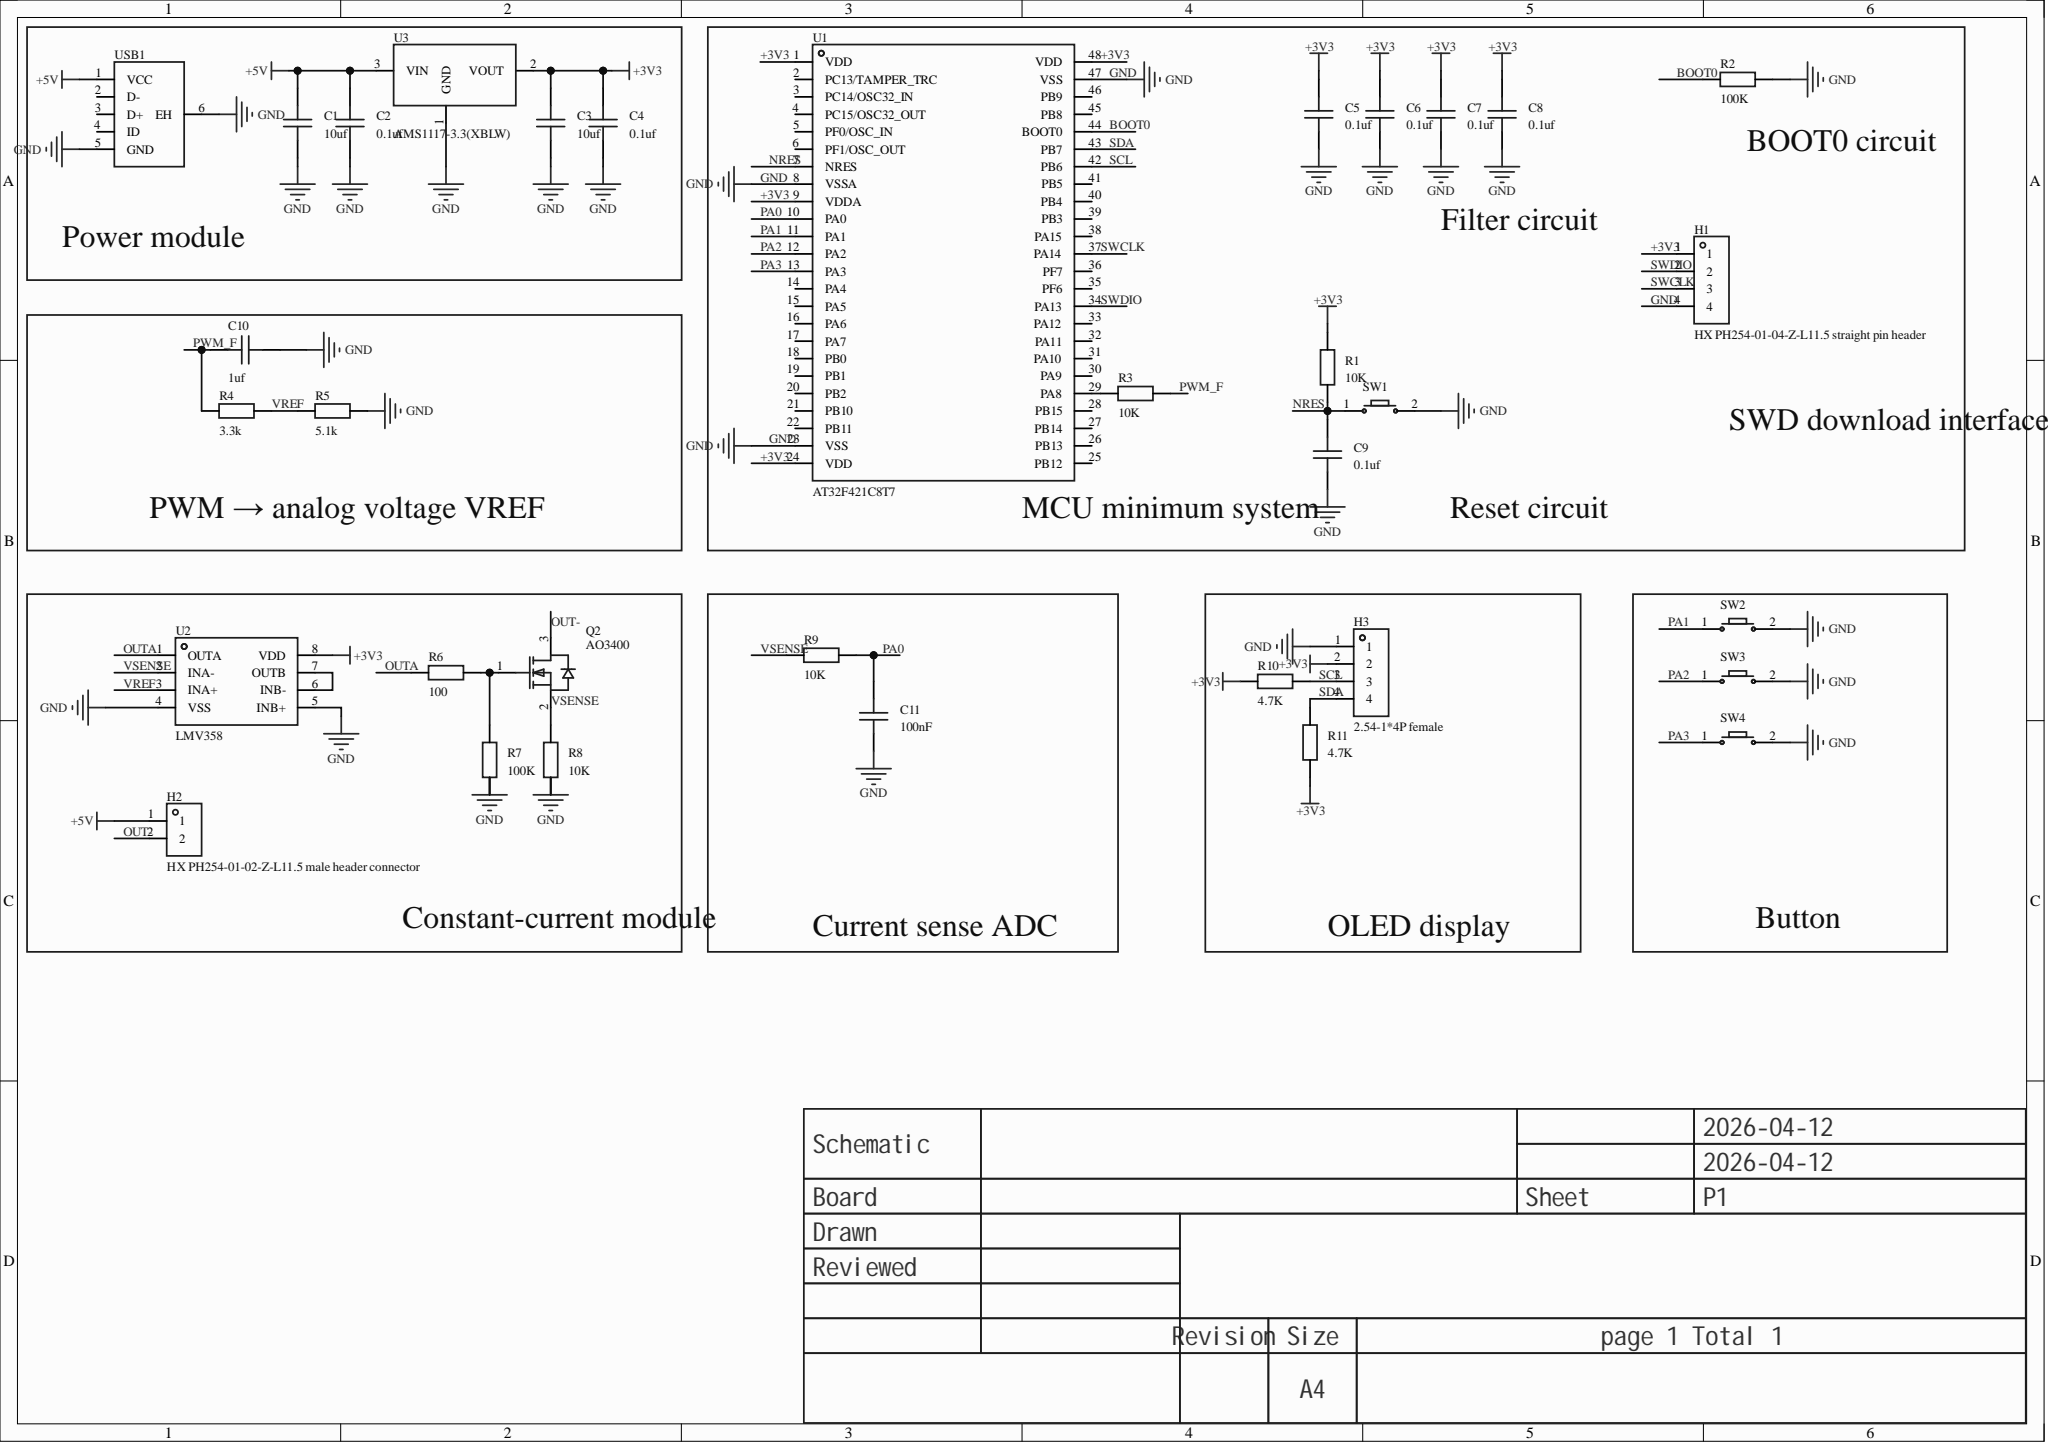Circuit board | Altium Designer | 34 parts | 21 nets
Bill of materials:
Comment,Description,Designator,Footprint,LibRef,Quantity
"10uf","","C1, C3","C0603","CAP_0603","2"
"0.1uf","","C2, C4, C5, C6, C7, C8, C9","C0603","CAP_0603","7"
"1uf","","C10","C0603","CAP_0603","1"
"100nF","","C11","C0603","CAP_0603","1"
"HX PH254-01-04-Z-L11.5 straight pin header","插针结构:1x4P;间距:2.54mm;圆针/方针:方针;安装方式:直插;排数:单排;总PIN位数:4P;额定电流:3A;额定电压:1kV;配合针长度:6mm;塑高:2.5mm;端接针长度:3mm;触头材质:黄铜;触头镀层:金;工作温度:-40℃~+105℃;","H1","HDR-TH_4P-HX-PH254-01-04-Z-L11.5","HX PH254-01-04-Z-L11.5 straight pin header","1"
"HX PH254-01-02-Z-L11.5 male header connector","插针结构:1x2P;间距:2.54mm;圆针/方针:方针;安装方式:直插;排数:单排;总PIN位数:2P;额定电流:3A;额定电压:1kV;配合针长度:6mm;塑高:2.5mm;端接针长度:3mm;触头材质:黄铜;触头镀层:金;工作温度:-40℃~+105℃;","H2","HDR-TH_2P-P2.54-V-M","HX PH254-01-02-Z-L11.5 male header connector","1"
"2.54-1*4P female","插孔结构:1x4P;间距:2.54mm;行距:-;圆孔/方孔:方孔;安装方式:直插;排数:单排;总孔位数:4P;额定电流:3A;额定电压:-;插孔方向:顶部;塑高:-;触头材质:青铜;触头镀层:-;工作温度:-40℃~+105℃;","H3","HDR-TH_4P-P2.54-V-F","2.54-1*4P母","1"
"AO3400","","Q2","SOT-23_L2.9-W1.3-P1.90-LS2.4-BR","AO3400_C2938367","1"
"10K","","R1, R3, R8, R9","R0603","Res_0603","4"
"100K","","R2, R7","R0603","Res_0603","2"
"3.3k","","R4","R0603","Res_0603","1"
"5.1k","","R5","R0603","Res_0603","1"
"100","","R6","R0603","Res_0603","1"
"4.7K","","R10, R11","R0603","Res_0603","2"
"","","SW1, SW2, SW3, SW4","Key_SMD_3x4x2","Key_SMD_3x4x2","4"
"AT32F421C8T7","CPU内核:CM4;程序存储容量:64KB;RAM总容量:16KB;GPIO端口数量:-;工作电压范围:-;CPU最大主频:-;程序存储器类型:FLASH;","U1","LQFP-48_L7.0-W7.0-P0.50-LS9.0-BL","AT32F421C8T7","1"
"LMV358","放大器数:2;轨到轨:轨到轨输入,轨到轨输出;增益带宽积(GBW):1MHz;输入失调电压(Vos):5mV;压摆率(SR):600V/ms;输入偏置电流(Ib):10pA;","U2","SOP-8_L4.9-W3.9-P1.27-LS6.0-BL","LMV358","1"
"AMS1117-3.3(XBLW)","Output type: fixed; max input voltage: 15V; output voltage: 3.3V; output current: 1A; power supply rejection ratio (PSRR): 60dB; output polarity: positive;","U3","SOT-223-3_L6.5-W3.4-P2.30-LS7.0-BR-1","AMS1117-3.3(XBLW)","1"
"","","USB1","USB_Micro","USB_Micro-B","1"
Netlist (Protel format):
[
C1
C0603
10uf



]
[
C2
C0603
0.1uf



]
[
C3
C0603
10uf



]
[
C4
C0603
0.1uf



]
[
C5
C0603
0.1uf



]
[
C6
C0603
0.1uf



]
[
C7
C0603
0.1uf



]
[
C8
C0603
0.1uf



]
[
C9
C0603
0.1uf



]
[
C10
C0603
1uf



]
[
C11
C0603
100nF



]
[
H1
HDR-TH_4P-HX-PH254-01-04-Z-L11.5
HX PH254-01-04-Z-L11.5 straight pin header



]
[
H2
HDR-TH_2P-P2.54-V-M
HX PH254-01-02-Z-L11.5 male header connector



]
[
H3
HDR-TH_4P-P2.54-V-F
2.54-1*4P female



]
[
Q2
SOT-23_L2.9-W1.3-P1.90-LS2.4-BR
AO3400



]
[
R1
R0603
10K



]
[
R2
R0603
100K



]
[
R3
R0603
10K



]
[
R4
R0603
3.3k



]
[
R5
R0603
5.1k



]
[
R6
R0603
100



]
[
R7
R0603
100K



]
[
R8
R0603
10K



]
[
R9
R0603
10K



]
[
R10
R0603
4.7K



]
[
R11
R0603
4.7K



]
[
SW1
Key_SMD_3x4x2




]
[
SW2
Key_SMD_3x4x2




]
[
SW3
Key_SMD_3x4x2




]
[
SW4
Key_SMD_3x4x2




]
[
U1
LQFP-48_L7.0-W7.0-P0.50-LS9.0-BL
AT32F421C8T7



]
[
U2
SOP-8_L4.9-W3.9-P1.27-LS6.0-BL
LMV358



]
[
U3
SOT-223-3_L6.5-W3.4-P2.30-LS7.0-BR-1
AMS1117-3.3(XBLW)



]
[
USB1
USB_Micro




]
(
VSENSE
Q2-2
R8-2
R9-1
U2-2
)
(
VREF
R4-2
R5-1
U2-3
)
(
SWDIO
H1-2
U1-34
)
(
SWCLK
H1-3
U1-37
)
(
SDA
H3-4
R11-2
U1-43
)
(
SCL
H3-3
R10-2
U1-42
)
(
PWM_F
C10-1
R3-2
R4-1
)
(
PA3
SW4-1
U1-13
)
(
PA2
SW3-1
U1-12
)
(
PA1
SW2-1
U1-11
)
(
PA0
C11-2
R9-2
U1-10
)
(
OUTA
R6-1
U2-1
)
(
OUT-
H2-2
Q2-3
)
(
NRES
C9-2
R1-1
SW1-1
U1-7
)
(
NetU2_6
U2-6
U2-7
)
(
NetR3_1
R3-1
U1-29
)
(
NetQ2_1
Q2-1
R6-2
R7-2
)
(
GND
C1-1
C2-1
C3-1
C4-1
C5-1
C6-1
C7-1
C8-1
C9-1
C10-2
C11-1
H1-4
H3-1
R2-2
R5-2
R7-1
R8-1
SW1-2
SW2-2
SW3-2
SW4-2
U1-8
U1-23
U1-47
U2-4
U2-5
U3-1
USB1-5
USB1-6
)
(
BOOT0
R2-1
U1-44
)
(
+5V
C1-2
C2-2
H2-1
U3-3
USB1-1
)
(
+3V3
C3-2
C4-2
C5-2
C6-2
C7-2
C8-2
H1-1
H3-2
R1-2
R10-1
R11-1
U1-1
U1-9
U1-24
U1-48
U2-8
U3-2
)